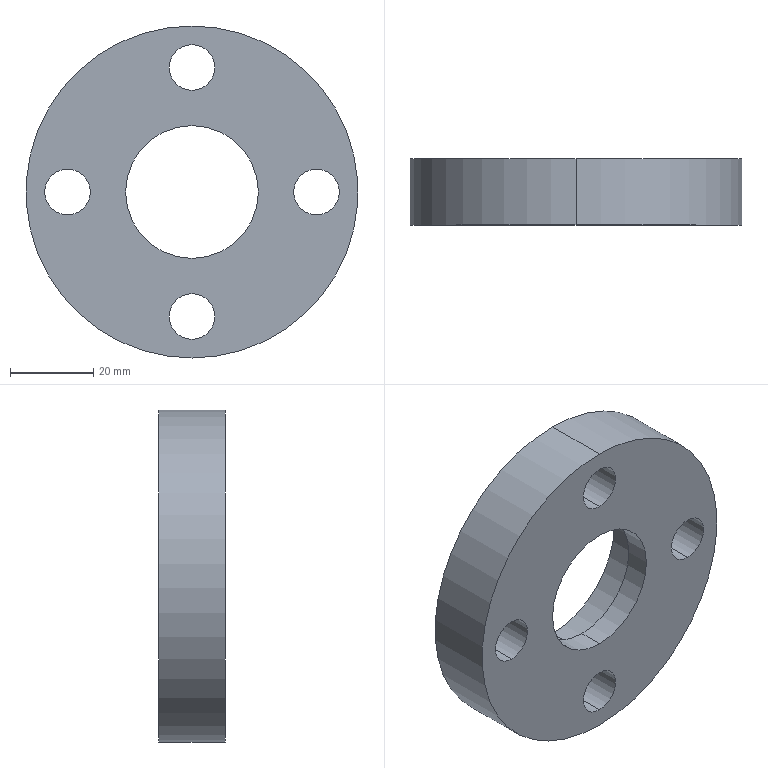Part | SolidWorks | features Extrusion 1, HoleWzd 1, ICE 1 | 1 solid | 17 faces | box 80 x 16 x 80 mm | volume 55663 mm3 | cylinder 14 | plane 3 | commonest cylinder face diameters 11 x8 32 x2 42 x2 80 x2
STEP:
#1=CARTESIAN_POINT('',(0.,0.,-35.5));
#2=VERTEX_POINT('',#1);
#3=CARTESIAN_POINT('',(0.,0.,-24.5));
#4=VERTEX_POINT('',#3);
#5=CARTESIAN_POINT('',(0.,0.,-30.));
#6=DIRECTION('',(0.,1.,0.));
#7=DIRECTION('',(0.,0.,1.));
#8=AXIS2_PLACEMENT_3D('',#5,#6,#7);
#9=CIRCLE('',#8,5.5);
#10=EDGE_CURVE('',#2,#4,#9,.T.);
#11=ORIENTED_EDGE('',*,*,#10,.F.);
#12=CARTESIAN_POINT('',(0.,16.,-35.5));
#13=VERTEX_POINT('',#12);
#14=CARTESIAN_POINT('',(0.,16.,-35.5));
#15=DIRECTION('',(0.,1.,0.));
#16=VECTOR('',#15,1000.);
#17=LINE('',#14,#16);
#18=EDGE_CURVE('',#2,#13,#17,.T.);
#19=ORIENTED_EDGE('',*,*,#18,.T.);
#20=CARTESIAN_POINT('',(0.,16.,-24.5));
#21=VERTEX_POINT('',#20);
#22=CARTESIAN_POINT('',(0.,16.,-30.));
#23=DIRECTION('',(0.,1.,0.));
#24=DIRECTION('',(0.,0.,1.));
#25=AXIS2_PLACEMENT_3D('',#22,#23,#24);
#26=CIRCLE('',#25,5.5);
#27=EDGE_CURVE('',#13,#21,#26,.T.);
#28=ORIENTED_EDGE('',*,*,#27,.T.);
#29=CARTESIAN_POINT('',(0.,16.,-24.5));
#30=DIRECTION('',(0.,1.,0.));
#31=VECTOR('',#30,1000.);
#32=LINE('',#29,#31);
#33=EDGE_CURVE('',#4,#21,#32,.T.);
#34=ORIENTED_EDGE('',*,*,#33,.F.);
#35=EDGE_LOOP('',(#11,#19,#28,#34));
#36=FACE_OUTER_BOUND('',#35,.T.);
#37=CARTESIAN_POINT('',(0.,16.,-30.));
#38=DIRECTION('',(0.,1.,0.));
#39=DIRECTION('',(0.,0.,1.));
#40=AXIS2_PLACEMENT_3D('',#37,#38,#39);
#41=CYLINDRICAL_SURFACE('',#40,5.5);
#42=ADVANCED_FACE('',(#36),#41,.F.);
#43=CARTESIAN_POINT('',(-30.,0.,-5.5));
#44=VERTEX_POINT('',#43);
#45=CARTESIAN_POINT('',(-30.,0.,5.5));
#46=VERTEX_POINT('',#45);
#47=CARTESIAN_POINT('',(-30.,0.,0.));
#48=DIRECTION('',(0.,1.,0.));
#49=DIRECTION('',(0.,0.,1.));
#50=AXIS2_PLACEMENT_3D('',#47,#48,#49);
#51=CIRCLE('',#50,5.5);
#52=EDGE_CURVE('',#44,#46,#51,.T.);
#53=ORIENTED_EDGE('',*,*,#52,.F.);
#54=CARTESIAN_POINT('',(-30.,16.,-5.5));
#55=VERTEX_POINT('',#54);
#56=CARTESIAN_POINT('',(-30.,16.,-5.5));
#57=DIRECTION('',(0.,1.,0.));
#58=VECTOR('',#57,1000.);
#59=LINE('',#56,#58);
#60=EDGE_CURVE('',#44,#55,#59,.T.);
#61=ORIENTED_EDGE('',*,*,#60,.T.);
#62=CARTESIAN_POINT('',(-30.,16.,5.5));
#63=VERTEX_POINT('',#62);
#64=CARTESIAN_POINT('',(-30.,16.,0.));
#65=DIRECTION('',(0.,1.,0.));
#66=DIRECTION('',(0.,0.,1.));
#67=AXIS2_PLACEMENT_3D('',#64,#65,#66);
#68=CIRCLE('',#67,5.5);
#69=EDGE_CURVE('',#55,#63,#68,.T.);
#70=ORIENTED_EDGE('',*,*,#69,.T.);
#71=CARTESIAN_POINT('',(-30.,16.,5.5));
#72=DIRECTION('',(0.,1.,0.));
#73=VECTOR('',#72,1000.);
#74=LINE('',#71,#73);
#75=EDGE_CURVE('',#46,#63,#74,.T.);
#76=ORIENTED_EDGE('',*,*,#75,.F.);
#77=EDGE_LOOP('',(#53,#61,#70,#76));
#78=FACE_OUTER_BOUND('',#77,.T.);
#79=CARTESIAN_POINT('',(-30.,16.,0.));
#80=DIRECTION('',(0.,1.,0.));
#81=DIRECTION('',(0.,0.,1.));
#82=AXIS2_PLACEMENT_3D('',#79,#80,#81);
#83=CYLINDRICAL_SURFACE('',#82,5.5);
#84=ADVANCED_FACE('',(#78),#83,.F.);
#85=CARTESIAN_POINT('',(30.,0.,-5.5));
#86=VERTEX_POINT('',#85);
#87=CARTESIAN_POINT('',(30.,0.,5.5));
#88=VERTEX_POINT('',#87);
#89=CARTESIAN_POINT('',(30.,0.,0.));
#90=DIRECTION('',(0.,1.,0.));
#91=DIRECTION('',(0.,0.,1.));
#92=AXIS2_PLACEMENT_3D('',#89,#90,#91);
#93=CIRCLE('',#92,5.5);
#94=EDGE_CURVE('',#86,#88,#93,.T.);
#95=ORIENTED_EDGE('',*,*,#94,.F.);
#96=CARTESIAN_POINT('',(30.,16.,-5.5));
#97=VERTEX_POINT('',#96);
#98=CARTESIAN_POINT('',(30.,16.,-5.5));
#99=DIRECTION('',(0.,1.,0.));
#100=VECTOR('',#99,1000.);
#101=LINE('',#98,#100);
#102=EDGE_CURVE('',#86,#97,#101,.T.);
#103=ORIENTED_EDGE('',*,*,#102,.T.);
#104=CARTESIAN_POINT('',(30.,16.,5.5));
#105=VERTEX_POINT('',#104);
#106=CARTESIAN_POINT('',(30.,16.,0.));
#107=DIRECTION('',(0.,1.,0.));
#108=DIRECTION('',(0.,0.,1.));
#109=AXIS2_PLACEMENT_3D('',#106,#107,#108);
#110=CIRCLE('',#109,5.5);
#111=EDGE_CURVE('',#97,#105,#110,.T.);
#112=ORIENTED_EDGE('',*,*,#111,.T.);
#113=CARTESIAN_POINT('',(30.,16.,5.5));
#114=DIRECTION('',(0.,1.,0.));
#115=VECTOR('',#114,1000.);
#116=LINE('',#113,#115);
#117=EDGE_CURVE('',#88,#105,#116,.T.);
#118=ORIENTED_EDGE('',*,*,#117,.F.);
#119=EDGE_LOOP('',(#95,#103,#112,#118));
#120=FACE_OUTER_BOUND('',#119,.T.);
#121=CARTESIAN_POINT('',(30.,16.,0.));
#122=DIRECTION('',(0.,1.,0.));
#123=DIRECTION('',(0.,0.,1.));
#124=AXIS2_PLACEMENT_3D('',#121,#122,#123);
#125=CYLINDRICAL_SURFACE('',#124,5.5);
#126=ADVANCED_FACE('',(#120),#125,.F.);
#127=CARTESIAN_POINT('',(0.,0.,24.5));
#128=VERTEX_POINT('',#127);
#129=CARTESIAN_POINT('',(0.,0.,35.5));
#130=VERTEX_POINT('',#129);
#131=CARTESIAN_POINT('',(0.,0.,30.));
#132=DIRECTION('',(0.,1.,0.));
#133=DIRECTION('',(0.,0.,1.));
#134=AXIS2_PLACEMENT_3D('',#131,#132,#133);
#135=CIRCLE('',#134,5.5);
#136=EDGE_CURVE('',#128,#130,#135,.T.);
#137=ORIENTED_EDGE('',*,*,#136,.F.);
#138=CARTESIAN_POINT('',(0.,16.,24.5));
#139=VERTEX_POINT('',#138);
#140=CARTESIAN_POINT('',(0.,16.,24.5));
#141=DIRECTION('',(0.,1.,0.));
#142=VECTOR('',#141,1000.);
#143=LINE('',#140,#142);
#144=EDGE_CURVE('',#128,#139,#143,.T.);
#145=ORIENTED_EDGE('',*,*,#144,.T.);
#146=CARTESIAN_POINT('',(0.,16.,35.5));
#147=VERTEX_POINT('',#146);
#148=CARTESIAN_POINT('',(0.,16.,30.));
#149=DIRECTION('',(0.,1.,0.));
#150=DIRECTION('',(0.,0.,1.));
#151=AXIS2_PLACEMENT_3D('',#148,#149,#150);
#152=CIRCLE('',#151,5.5);
#153=EDGE_CURVE('',#139,#147,#152,.T.);
#154=ORIENTED_EDGE('',*,*,#153,.T.);
#155=CARTESIAN_POINT('',(0.,16.,35.5));
#156=DIRECTION('',(0.,1.,0.));
#157=VECTOR('',#156,1000.);
#158=LINE('',#155,#157);
#159=EDGE_CURVE('',#130,#147,#158,.T.);
#160=ORIENTED_EDGE('',*,*,#159,.F.);
#161=EDGE_LOOP('',(#137,#145,#154,#160));
#162=FACE_OUTER_BOUND('',#161,.T.);
#163=CARTESIAN_POINT('',(0.,16.,30.));
#164=DIRECTION('',(0.,1.,0.));
#165=DIRECTION('',(0.,0.,1.));
#166=AXIS2_PLACEMENT_3D('',#163,#164,#165);
#167=CYLINDRICAL_SURFACE('',#166,5.5);
#168=ADVANCED_FACE('',(#162),#167,.F.);
#169=CARTESIAN_POINT('',(0.,6.,-21.));
#170=VERTEX_POINT('',#169);
#171=CARTESIAN_POINT('',(0.,6.,21.));
#172=VERTEX_POINT('',#171);
#173=CARTESIAN_POINT('',(0.,6.,0.));
#174=DIRECTION('',(0.,1.,0.));
#175=DIRECTION('',(0.,0.,1.));
#176=AXIS2_PLACEMENT_3D('',#173,#174,#175);
#177=CIRCLE('',#176,21.);
#178=EDGE_CURVE('',#170,#172,#177,.T.);
#179=ORIENTED_EDGE('',*,*,#178,.F.);
#180=CARTESIAN_POINT('',(0.,16.,-21.));
#181=VERTEX_POINT('',#180);
#182=CARTESIAN_POINT('',(0.,6.,-21.));
#183=DIRECTION('',(0.,1.,0.));
#184=VECTOR('',#183,1000.);
#185=LINE('',#182,#184);
#186=EDGE_CURVE('',#170,#181,#185,.T.);
#187=ORIENTED_EDGE('',*,*,#186,.T.);
#188=CARTESIAN_POINT('',(0.,16.,21.));
#189=VERTEX_POINT('',#188);
#190=CARTESIAN_POINT('',(0.,16.,0.));
#191=DIRECTION('',(0.,1.,0.));
#192=DIRECTION('',(0.,0.,1.));
#193=AXIS2_PLACEMENT_3D('',#190,#191,#192);
#194=CIRCLE('',#193,21.);
#195=EDGE_CURVE('',#181,#189,#194,.T.);
#196=ORIENTED_EDGE('',*,*,#195,.T.);
#197=CARTESIAN_POINT('',(0.,6.,21.));
#198=DIRECTION('',(0.,1.,0.));
#199=VECTOR('',#198,1000.);
#200=LINE('',#197,#199);
#201=EDGE_CURVE('',#172,#189,#200,.T.);
#202=ORIENTED_EDGE('',*,*,#201,.F.);
#203=EDGE_LOOP('',(#179,#187,#196,#202));
#204=FACE_OUTER_BOUND('',#203,.T.);
#205=CARTESIAN_POINT('',(0.,6.,0.));
#206=DIRECTION('',(0.,1.,0.));
#207=DIRECTION('',(0.,0.,1.));
#208=AXIS2_PLACEMENT_3D('',#205,#206,#207);
#209=CYLINDRICAL_SURFACE('',#208,21.);
#210=ADVANCED_FACE('',(#204),#209,.F.);
#211=CARTESIAN_POINT('',(0.,16.,40.));
#212=VERTEX_POINT('',#211);
#213=CARTESIAN_POINT('',(0.,16.,-40.));
#214=VERTEX_POINT('',#213);
#215=CARTESIAN_POINT('',(0.,16.,0.));
#216=DIRECTION('',(0.,1.,0.));
#217=DIRECTION('',(0.,0.,1.));
#218=AXIS2_PLACEMENT_3D('',#215,#216,#217);
#219=CIRCLE('',#218,40.);
#220=EDGE_CURVE('',#212,#214,#219,.T.);
#221=ORIENTED_EDGE('',*,*,#220,.F.);
#222=CARTESIAN_POINT('',(0.,0.,40.));
#223=VERTEX_POINT('',#222);
#224=CARTESIAN_POINT('',(0.,16.,40.));
#225=DIRECTION('',(0.,-1.,0.));
#226=VECTOR('',#225,1000.);
#227=LINE('',#224,#226);
#228=EDGE_CURVE('',#212,#223,#227,.T.);
#229=ORIENTED_EDGE('',*,*,#228,.T.);
#230=CARTESIAN_POINT('',(0.,0.,-40.));
#231=VERTEX_POINT('',#230);
#232=CARTESIAN_POINT('',(0.,0.,0.));
#233=DIRECTION('',(0.,1.,0.));
#234=DIRECTION('',(0.,0.,1.));
#235=AXIS2_PLACEMENT_3D('',#232,#233,#234);
#236=CIRCLE('',#235,40.);
#237=EDGE_CURVE('',#223,#231,#236,.T.);
#238=ORIENTED_EDGE('',*,*,#237,.T.);
#239=CARTESIAN_POINT('',(0.,16.,-40.));
#240=DIRECTION('',(0.,-1.,0.));
#241=VECTOR('',#240,1000.);
#242=LINE('',#239,#241);
#243=EDGE_CURVE('',#214,#231,#242,.T.);
#244=ORIENTED_EDGE('',*,*,#243,.F.);
#245=EDGE_LOOP('',(#221,#229,#238,#244));
#246=FACE_OUTER_BOUND('',#245,.T.);
#247=CARTESIAN_POINT('',(0.,16.,0.));
#248=DIRECTION('',(0.,-1.,0.));
#249=DIRECTION('',(0.,0.,-1.));
#250=AXIS2_PLACEMENT_3D('',#247,#248,#249);
#251=CYLINDRICAL_SURFACE('',#250,40.);
#252=ADVANCED_FACE('',(#246),#251,.T.);
#253=CARTESIAN_POINT('',(0.,6.,-16.));
#254=VERTEX_POINT('',#253);
#255=CARTESIAN_POINT('',(0.,6.,16.));
#256=VERTEX_POINT('',#255);
#257=CARTESIAN_POINT('',(0.,6.,0.));
#258=DIRECTION('',(0.,1.,0.));
#259=DIRECTION('',(0.,0.,1.));
#260=AXIS2_PLACEMENT_3D('',#257,#258,#259);
#261=CIRCLE('',#260,16.);
#262=EDGE_CURVE('',#254,#256,#261,.T.);
#263=ORIENTED_EDGE('',*,*,#262,.T.);
#264=CARTESIAN_POINT('',(0.,0.,16.));
#265=VERTEX_POINT('',#264);
#266=CARTESIAN_POINT('',(0.,16.,16.));
#267=DIRECTION('',(0.,-1.,0.));
#268=VECTOR('',#267,1000.);
#269=LINE('',#266,#268);
#270=EDGE_CURVE('',#256,#265,#269,.T.);
#271=ORIENTED_EDGE('',*,*,#270,.T.);
#272=CARTESIAN_POINT('',(0.,0.,-16.));
#273=VERTEX_POINT('',#272);
#274=CARTESIAN_POINT('',(0.,0.,0.));
#275=DIRECTION('',(0.,1.,0.));
#276=DIRECTION('',(0.,0.,1.));
#277=AXIS2_PLACEMENT_3D('',#274,#275,#276);
#278=CIRCLE('',#277,16.);
#279=EDGE_CURVE('',#273,#265,#278,.T.);
#280=ORIENTED_EDGE('',*,*,#279,.F.);
#281=CARTESIAN_POINT('',(0.,16.,-16.));
#282=DIRECTION('',(0.,-1.,0.));
#283=VECTOR('',#282,1000.);
#284=LINE('',#281,#283);
#285=EDGE_CURVE('',#254,#273,#284,.T.);
#286=ORIENTED_EDGE('',*,*,#285,.F.);
#287=EDGE_LOOP('',(#263,#271,#280,#286));
#288=FACE_OUTER_BOUND('',#287,.T.);
#289=CARTESIAN_POINT('',(0.,16.,0.));
#290=DIRECTION('',(0.,-1.,0.));
#291=DIRECTION('',(0.,0.,-1.));
#292=AXIS2_PLACEMENT_3D('',#289,#290,#291);
#293=CYLINDRICAL_SURFACE('',#292,16.);
#294=ADVANCED_FACE('',(#288),#293,.F.);
#295=ORIENTED_EDGE('',*,*,#270,.F.);
#296=CARTESIAN_POINT('',(0.,6.,0.));
#297=DIRECTION('',(0.,1.,0.));
#298=DIRECTION('',(0.,0.,1.));
#299=AXIS2_PLACEMENT_3D('',#296,#297,#298);
#300=CIRCLE('',#299,16.);
#301=EDGE_CURVE('',#256,#254,#300,.T.);
#302=ORIENTED_EDGE('',*,*,#301,.T.);
#303=ORIENTED_EDGE('',*,*,#285,.T.);
#304=CARTESIAN_POINT('',(0.,0.,0.));
#305=DIRECTION('',(0.,1.,0.));
#306=DIRECTION('',(0.,0.,1.));
#307=AXIS2_PLACEMENT_3D('',#304,#305,#306);
#308=CIRCLE('',#307,16.);
#309=EDGE_CURVE('',#265,#273,#308,.T.);
#310=ORIENTED_EDGE('',*,*,#309,.F.);
#311=EDGE_LOOP('',(#295,#302,#303,#310));
#312=FACE_OUTER_BOUND('',#311,.T.);
#313=CARTESIAN_POINT('',(0.,16.,0.));
#314=DIRECTION('',(0.,-1.,0.));
#315=DIRECTION('',(0.,0.,-1.));
#316=AXIS2_PLACEMENT_3D('',#313,#314,#315);
#317=CYLINDRICAL_SURFACE('',#316,16.);
#318=ADVANCED_FACE('',(#312),#317,.F.);
#319=CARTESIAN_POINT('',(0.,16.,-30.));
#320=DIRECTION('',(0.,1.,0.));
#321=DIRECTION('',(0.,0.,1.));
#322=AXIS2_PLACEMENT_3D('',#319,#320,#321);
#323=CIRCLE('',#322,5.5);
#324=EDGE_CURVE('',#21,#13,#323,.T.);
#325=ORIENTED_EDGE('',*,*,#324,.F.);
#326=ORIENTED_EDGE('',*,*,#27,.F.);
#327=EDGE_LOOP('',(#325,#326));
#328=FACE_BOUND('',#327,.T.);
#329=CARTESIAN_POINT('',(-30.,16.,0.));
#330=DIRECTION('',(0.,1.,0.));
#331=DIRECTION('',(0.,0.,1.));
#332=AXIS2_PLACEMENT_3D('',#329,#330,#331);
#333=CIRCLE('',#332,5.5);
#334=EDGE_CURVE('',#63,#55,#333,.T.);
#335=ORIENTED_EDGE('',*,*,#334,.F.);
#336=ORIENTED_EDGE('',*,*,#69,.F.);
#337=EDGE_LOOP('',(#335,#336));
#338=FACE_BOUND('',#337,.T.);
#339=CARTESIAN_POINT('',(30.,16.,0.));
#340=DIRECTION('',(0.,1.,0.));
#341=DIRECTION('',(0.,0.,1.));
#342=AXIS2_PLACEMENT_3D('',#339,#340,#341);
#343=CIRCLE('',#342,5.5);
#344=EDGE_CURVE('',#105,#97,#343,.T.);
#345=ORIENTED_EDGE('',*,*,#344,.F.);
#346=ORIENTED_EDGE('',*,*,#111,.F.);
#347=EDGE_LOOP('',(#345,#346));
#348=FACE_BOUND('',#347,.T.);
#349=CARTESIAN_POINT('',(0.,16.,30.));
#350=DIRECTION('',(0.,1.,0.));
#351=DIRECTION('',(0.,0.,1.));
#352=AXIS2_PLACEMENT_3D('',#349,#350,#351);
#353=CIRCLE('',#352,5.5);
#354=EDGE_CURVE('',#147,#139,#353,.T.);
#355=ORIENTED_EDGE('',*,*,#354,.F.);
#356=ORIENTED_EDGE('',*,*,#153,.F.);
#357=EDGE_LOOP('',(#355,#356));
#358=FACE_BOUND('',#357,.T.);
#359=CARTESIAN_POINT('',(0.,16.,0.));
#360=DIRECTION('',(0.,1.,0.));
#361=DIRECTION('',(0.,0.,1.));
#362=AXIS2_PLACEMENT_3D('',#359,#360,#361);
#363=CIRCLE('',#362,21.);
#364=EDGE_CURVE('',#189,#181,#363,.T.);
#365=ORIENTED_EDGE('',*,*,#364,.F.);
#366=ORIENTED_EDGE('',*,*,#195,.F.);
#367=EDGE_LOOP('',(#365,#366));
#368=FACE_BOUND('',#367,.T.);
#369=CARTESIAN_POINT('',(0.,16.,0.));
#370=DIRECTION('',(0.,1.,0.));
#371=DIRECTION('',(0.,0.,1.));
#372=AXIS2_PLACEMENT_3D('',#369,#370,#371);
#373=CIRCLE('',#372,40.);
#374=EDGE_CURVE('',#214,#212,#373,.T.);
#375=ORIENTED_EDGE('',*,*,#374,.T.);
#376=ORIENTED_EDGE('',*,*,#220,.T.);
#377=EDGE_LOOP('',(#375,#376));
#378=FACE_OUTER_BOUND('',#377,.T.);
#379=CARTESIAN_POINT('',(0.,16.,0.));
#380=DIRECTION('',(0.,1.,0.));
#381=DIRECTION('',(0.,0.,1.));
#382=AXIS2_PLACEMENT_3D('',#379,#380,#381);
#383=PLANE('',#382);
#384=ADVANCED_FACE('',(#328,#338,#348,#358,#368,#378),#383,.T.);
#385=CARTESIAN_POINT('',(0.,0.,-30.));
#386=DIRECTION('',(0.,1.,0.));
#387=DIRECTION('',(0.,0.,1.));
#388=AXIS2_PLACEMENT_3D('',#385,#386,#387);
#389=CIRCLE('',#388,5.5);
#390=EDGE_CURVE('',#4,#2,#389,.T.);
#391=ORIENTED_EDGE('',*,*,#390,.T.);
#392=ORIENTED_EDGE('',*,*,#10,.T.);
#393=EDGE_LOOP('',(#391,#392));
#394=FACE_BOUND('',#393,.T.);
#395=CARTESIAN_POINT('',(-30.,0.,0.));
#396=DIRECTION('',(0.,1.,0.));
#397=DIRECTION('',(0.,0.,1.));
#398=AXIS2_PLACEMENT_3D('',#395,#396,#397);
#399=CIRCLE('',#398,5.5);
#400=EDGE_CURVE('',#46,#44,#399,.T.);
#401=ORIENTED_EDGE('',*,*,#400,.T.);
#402=ORIENTED_EDGE('',*,*,#52,.T.);
#403=EDGE_LOOP('',(#401,#402));
#404=FACE_BOUND('',#403,.T.);
#405=CARTESIAN_POINT('',(30.,0.,0.));
#406=DIRECTION('',(0.,1.,0.));
#407=DIRECTION('',(0.,0.,1.));
#408=AXIS2_PLACEMENT_3D('',#405,#406,#407);
#409=CIRCLE('',#408,5.5);
#410=EDGE_CURVE('',#88,#86,#409,.T.);
#411=ORIENTED_EDGE('',*,*,#410,.T.);
#412=ORIENTED_EDGE('',*,*,#94,.T.);
#413=EDGE_LOOP('',(#411,#412));
#414=FACE_BOUND('',#413,.T.);
#415=CARTESIAN_POINT('',(0.,0.,30.));
#416=DIRECTION('',(0.,1.,0.));
#417=DIRECTION('',(0.,0.,1.));
#418=AXIS2_PLACEMENT_3D('',#415,#416,#417);
#419=CIRCLE('',#418,5.5);
#420=EDGE_CURVE('',#130,#128,#419,.T.);
#421=ORIENTED_EDGE('',*,*,#420,.T.);
#422=ORIENTED_EDGE('',*,*,#136,.T.);
#423=EDGE_LOOP('',(#421,#422));
#424=FACE_BOUND('',#423,.T.);
#425=CARTESIAN_POINT('',(0.,0.,0.));
#426=DIRECTION('',(0.,1.,0.));
#427=DIRECTION('',(0.,0.,1.));
#428=AXIS2_PLACEMENT_3D('',#425,#426,#427);
#429=CIRCLE('',#428,40.);
#430=EDGE_CURVE('',#231,#223,#429,.T.);
#431=ORIENTED_EDGE('',*,*,#430,.F.);
#432=ORIENTED_EDGE('',*,*,#237,.F.);
#433=EDGE_LOOP('',(#431,#432));
#434=FACE_OUTER_BOUND('',#433,.T.);
#435=ORIENTED_EDGE('',*,*,#279,.T.);
#436=ORIENTED_EDGE('',*,*,#309,.T.);
#437=EDGE_LOOP('',(#435,#436));
#438=FACE_BOUND('',#437,.T.);
#439=CARTESIAN_POINT('',(0.,0.,0.));
#440=DIRECTION('',(0.,1.,0.));
#441=DIRECTION('',(0.,0.,1.));
#442=AXIS2_PLACEMENT_3D('',#439,#440,#441);
#443=PLANE('',#442);
#444=ADVANCED_FACE('',(#394,#404,#414,#424,#434,#438),#443,.F.);
#445=ORIENTED_EDGE('',*,*,#228,.F.);
#446=ORIENTED_EDGE('',*,*,#374,.F.);
#447=ORIENTED_EDGE('',*,*,#243,.T.);
#448=ORIENTED_EDGE('',*,*,#430,.T.);
#449=EDGE_LOOP('',(#445,#446,#447,#448));
#450=FACE_OUTER_BOUND('',#449,.T.);
#451=CARTESIAN_POINT('',(0.,16.,0.));
#452=DIRECTION('',(0.,-1.,0.));
#453=DIRECTION('',(0.,0.,-1.));
#454=AXIS2_PLACEMENT_3D('',#451,#452,#453);
#455=CYLINDRICAL_SURFACE('',#454,40.);
#456=ADVANCED_FACE('',(#450),#455,.T.);
#457=ORIENTED_EDGE('',*,*,#186,.F.);
#458=CARTESIAN_POINT('',(0.,6.,0.));
#459=DIRECTION('',(0.,1.,0.));
#460=DIRECTION('',(0.,0.,1.));
#461=AXIS2_PLACEMENT_3D('',#458,#459,#460);
#462=CIRCLE('',#461,21.);
#463=EDGE_CURVE('',#172,#170,#462,.T.);
#464=ORIENTED_EDGE('',*,*,#463,.F.);
#465=ORIENTED_EDGE('',*,*,#201,.T.);
#466=ORIENTED_EDGE('',*,*,#364,.T.);
#467=EDGE_LOOP('',(#457,#464,#465,#466));
#468=FACE_OUTER_BOUND('',#467,.T.);
#469=CARTESIAN_POINT('',(0.,6.,0.));
#470=DIRECTION('',(0.,1.,0.));
#471=DIRECTION('',(0.,0.,1.));
#472=AXIS2_PLACEMENT_3D('',#469,#470,#471);
#473=CYLINDRICAL_SURFACE('',#472,21.);
#474=ADVANCED_FACE('',(#468),#473,.F.);
#475=ORIENTED_EDGE('',*,*,#262,.F.);
#476=ORIENTED_EDGE('',*,*,#301,.F.);
#477=EDGE_LOOP('',(#475,#476));
#478=FACE_BOUND('',#477,.T.);
#479=ORIENTED_EDGE('',*,*,#463,.T.);
#480=ORIENTED_EDGE('',*,*,#178,.T.);
#481=EDGE_LOOP('',(#479,#480));
#482=FACE_OUTER_BOUND('',#481,.T.);
#483=CARTESIAN_POINT('',(0.,6.,0.));
#484=DIRECTION('',(0.,1.,0.));
#485=DIRECTION('',(0.,0.,1.));
#486=AXIS2_PLACEMENT_3D('',#483,#484,#485);
#487=PLANE('',#486);
#488=ADVANCED_FACE('',(#478,#482),#487,.T.);
#489=ORIENTED_EDGE('',*,*,#144,.F.);
#490=ORIENTED_EDGE('',*,*,#420,.F.);
#491=ORIENTED_EDGE('',*,*,#159,.T.);
#492=ORIENTED_EDGE('',*,*,#354,.T.);
#493=EDGE_LOOP('',(#489,#490,#491,#492));
#494=FACE_OUTER_BOUND('',#493,.T.);
#495=CARTESIAN_POINT('',(0.,16.,30.));
#496=DIRECTION('',(0.,1.,0.));
#497=DIRECTION('',(0.,0.,1.));
#498=AXIS2_PLACEMENT_3D('',#495,#496,#497);
#499=CYLINDRICAL_SURFACE('',#498,5.5);
#500=ADVANCED_FACE('',(#494),#499,.F.);
#501=ORIENTED_EDGE('',*,*,#102,.F.);
#502=ORIENTED_EDGE('',*,*,#410,.F.);
#503=ORIENTED_EDGE('',*,*,#117,.T.);
#504=ORIENTED_EDGE('',*,*,#344,.T.);
#505=EDGE_LOOP('',(#501,#502,#503,#504));
#506=FACE_OUTER_BOUND('',#505,.T.);
#507=CARTESIAN_POINT('',(30.,16.,0.));
#508=DIRECTION('',(0.,1.,0.));
#509=DIRECTION('',(0.,0.,1.));
#510=AXIS2_PLACEMENT_3D('',#507,#508,#509);
#511=CYLINDRICAL_SURFACE('',#510,5.5);
#512=ADVANCED_FACE('',(#506),#511,.F.);
#513=ORIENTED_EDGE('',*,*,#60,.F.);
#514=ORIENTED_EDGE('',*,*,#400,.F.);
#515=ORIENTED_EDGE('',*,*,#75,.T.);
#516=ORIENTED_EDGE('',*,*,#334,.T.);
#517=EDGE_LOOP('',(#513,#514,#515,#516));
#518=FACE_OUTER_BOUND('',#517,.T.);
#519=CARTESIAN_POINT('',(-30.,16.,0.));
#520=DIRECTION('',(0.,1.,0.));
#521=DIRECTION('',(0.,0.,1.));
#522=AXIS2_PLACEMENT_3D('',#519,#520,#521);
#523=CYLINDRICAL_SURFACE('',#522,5.5);
#524=ADVANCED_FACE('',(#518),#523,.F.);
#525=ORIENTED_EDGE('',*,*,#18,.F.);
#526=ORIENTED_EDGE('',*,*,#390,.F.);
#527=ORIENTED_EDGE('',*,*,#33,.T.);
#528=ORIENTED_EDGE('',*,*,#324,.T.);
#529=EDGE_LOOP('',(#525,#526,#527,#528));
#530=FACE_OUTER_BOUND('',#529,.T.);
#531=CARTESIAN_POINT('',(0.,16.,-30.));
#532=DIRECTION('',(0.,1.,0.));
#533=DIRECTION('',(0.,0.,1.));
#534=AXIS2_PLACEMENT_3D('',#531,#532,#533);
#535=CYLINDRICAL_SURFACE('',#534,5.5);
#536=ADVANCED_FACE('',(#530),#535,.F.);
#537=CLOSED_SHELL('',(#42,#84,#126,#168,#210,#252,#294,#318,#384,#444,#456,#474,#488,#500,#512,#524,#536));
#538=MANIFOLD_SOLID_BREP('',#537);
#539=CARTESIAN_POINT('',(0.,0.,0.));
#540=DIRECTION('',(0.,0.,1.));
#541=DIRECTION('',(1.,0.,0.));
#542=AXIS2_PLACEMENT_3D('',#539,#540,#541);
#543=(LENGTH_UNIT()NAMED_UNIT(*)SI_UNIT(.MILLI.,.METRE.));
#544=UNCERTAINTY_MEASURE_WITH_UNIT(LENGTH_MEASURE(0.00001),#543,'','');
#545=(NAMED_UNIT(*)PLANE_ANGLE_UNIT()SI_UNIT($,.RADIAN.));
#546=(NAMED_UNIT(*)SI_UNIT($,.STERADIAN.)SOLID_ANGLE_UNIT());
#547=(GEOMETRIC_REPRESENTATION_CONTEXT(3)GLOBAL_UNCERTAINTY_ASSIGNED_CONTEXT((#544))GLOBAL_UNIT_ASSIGNED_CONTEXT((#543,#545,#546))REPRESENTATION_CONTEXT('',''));
#548=ADVANCED_BREP_SHAPE_REPRESENTATION('',(#538,#542),#547);